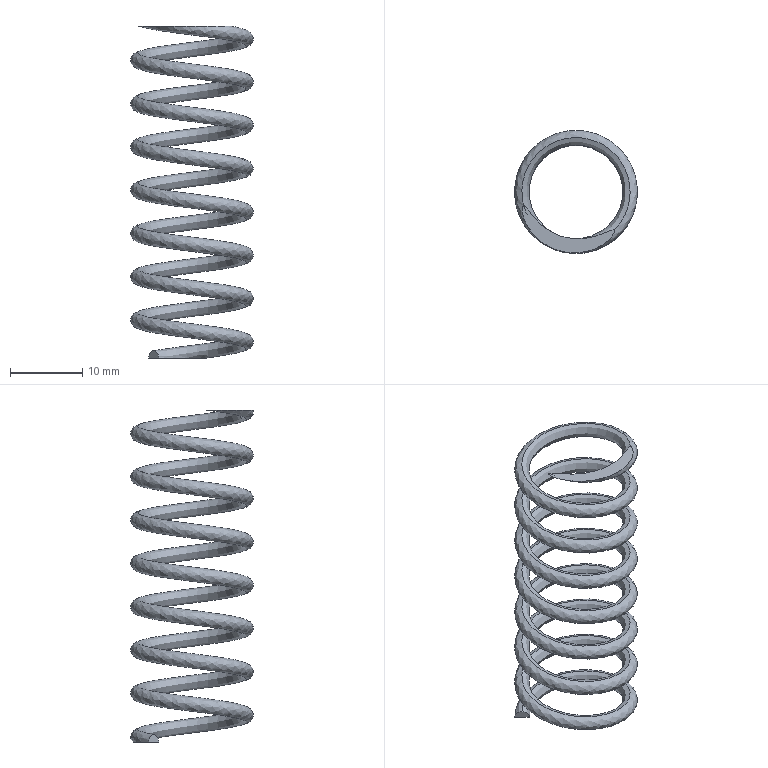Part | SolidWorks | features Helix 1, ICE 1, Sweep 1 | 1 solid | 5 faces | box 17 x 17 x 46 mm | volume 1130 mm3 | plane 3 | spline 2